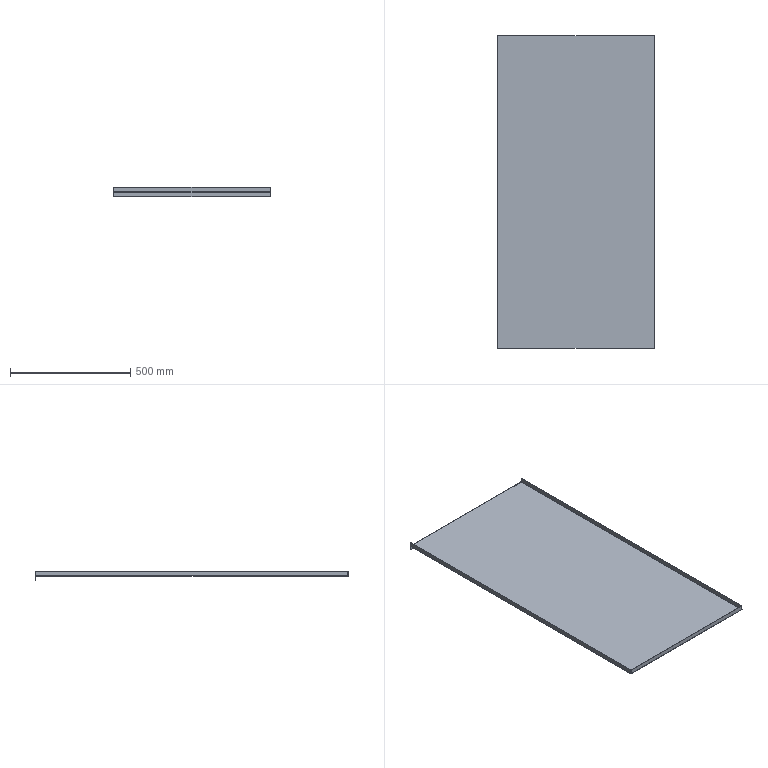Part | SolidWorks | 1 solid | 38 faces | box 655.001 x 1302 x 38.5 mm | volume 1385254 mm3 | plane 26 | cylinder 8 | spline 4 | commonest cylinder face diameters 0.2 x4 3.2 x4
STEP:
#1=CARTESIAN_POINT('',(325.9,-649.4,-1.5));
#2=VERTEX_POINT('',#1);
#3=CARTESIAN_POINT('',(-325.9,-649.4,-1.5));
#4=VERTEX_POINT('',#3);
#5=CARTESIAN_POINT('',(325.9,-649.4,-1.5));
#6=DIRECTION('',(-1.,0.,0.));
#7=VECTOR('',#6,1000.);
#8=LINE('',#5,#7);
#9=EDGE_CURVE('',#2,#4,#8,.T.);
#10=ORIENTED_EDGE('',*,*,#9,.T.);
#11=CARTESIAN_POINT('',(-325.9,649.4,-1.5));
#12=VERTEX_POINT('',#11);
#13=CARTESIAN_POINT('',(-325.9,-649.4,-1.5));
#14=DIRECTION('',(0.,1.,0.));
#15=VECTOR('',#14,1000.);
#16=LINE('',#13,#15);
#17=EDGE_CURVE('',#4,#12,#16,.T.);
#18=ORIENTED_EDGE('',*,*,#17,.T.);
#19=CARTESIAN_POINT('',(325.9,649.4,-1.5));
#20=VERTEX_POINT('',#19);
#21=CARTESIAN_POINT('',(325.9,649.4,-1.5));
#22=DIRECTION('',(-1.,0.,0.));
#23=VECTOR('',#22,1000.);
#24=LINE('',#21,#23);
#25=EDGE_CURVE('',#20,#12,#24,.T.);
#26=ORIENTED_EDGE('',*,*,#25,.F.);
#27=CARTESIAN_POINT('',(325.9,649.4,-1.5));
#28=DIRECTION('',(0.,-1.,0.));
#29=VECTOR('',#28,1000.);
#30=LINE('',#27,#29);
#31=EDGE_CURVE('',#20,#2,#30,.T.);
#32=ORIENTED_EDGE('',*,*,#31,.T.);
#33=EDGE_LOOP('',(#10,#18,#26,#32));
#34=FACE_OUTER_BOUND('',#33,.T.);
#35=CARTESIAN_POINT('',(0.,0.,-1.5));
#36=DIRECTION('',(0.,0.,1.));
#37=DIRECTION('',(1.,0.,0.));
#38=AXIS2_PLACEMENT_3D('',#35,#36,#37);
#39=PLANE('',#38);
#40=ADVANCED_FACE('',(#34),#39,.F.);
#41=CARTESIAN_POINT('',(-325.9,-649.4,0.));
#42=VERTEX_POINT('',#41);
#43=CARTESIAN_POINT('',(-325.9,649.4,0.));
#44=VERTEX_POINT('',#43);
#45=CARTESIAN_POINT('',(-325.9,-649.4,0.));
#46=DIRECTION('',(0.,1.,0.));
#47=VECTOR('',#46,1000.);
#48=LINE('',#45,#47);
#49=EDGE_CURVE('',#42,#44,#48,.T.);
#50=ORIENTED_EDGE('',*,*,#49,.F.);
#51=CARTESIAN_POINT('',(325.9,-649.4,0.));
#52=VERTEX_POINT('',#51);
#53=CARTESIAN_POINT('',(325.9,-649.4,0.));
#54=DIRECTION('',(-1.,0.,0.));
#55=VECTOR('',#54,1000.);
#56=LINE('',#53,#55);
#57=EDGE_CURVE('',#52,#42,#56,.T.);
#58=ORIENTED_EDGE('',*,*,#57,.F.);
#59=CARTESIAN_POINT('',(325.9,649.4,0.));
#60=VERTEX_POINT('',#59);
#61=CARTESIAN_POINT('',(325.9,649.4,0.));
#62=DIRECTION('',(0.,-1.,0.));
#63=VECTOR('',#62,1000.);
#64=LINE('',#61,#63);
#65=EDGE_CURVE('',#60,#52,#64,.T.);
#66=ORIENTED_EDGE('',*,*,#65,.F.);
#67=CARTESIAN_POINT('',(325.9,649.4,0.));
#68=DIRECTION('',(-1.,0.,0.));
#69=VECTOR('',#68,1000.);
#70=LINE('',#67,#69);
#71=EDGE_CURVE('',#60,#44,#70,.T.);
#72=ORIENTED_EDGE('',*,*,#71,.T.);
#73=EDGE_LOOP('',(#50,#58,#66,#72));
#74=FACE_OUTER_BOUND('',#73,.T.);
#75=CARTESIAN_POINT('',(0.,0.,0.));
#76=DIRECTION('',(0.,0.,1.));
#77=DIRECTION('',(1.,0.,0.));
#78=AXIS2_PLACEMENT_3D('',#75,#76,#77);
#79=PLANE('',#78);
#80=ADVANCED_FACE('',(#74),#79,.T.);
#81=CARTESIAN_POINT('',(-327.5,649.4,0.1));
#82=VERTEX_POINT('',#81);
#83=CARTESIAN_POINT('',(-326.,649.4,0.1));
#84=VERTEX_POINT('',#83);
#85=CARTESIAN_POINT('',(-326.,649.4,0.1));
#86=DIRECTION('',(1.,0.,0.));
#87=VECTOR('',#86,1000.);
#88=LINE('',#85,#87);
#89=EDGE_CURVE('',#82,#84,#88,.T.);
#90=ORIENTED_EDGE('',*,*,#89,.T.);
#91=CARTESIAN_POINT('',(-325.9,649.4,0.1));
#92=DIRECTION('',(0.,1.,0.));
#93=DIRECTION('',(0.,0.,-1.));
#94=AXIS2_PLACEMENT_3D('',#91,#92,#93);
#95=CIRCLE('',#94,0.1);
#96=EDGE_CURVE('',#44,#84,#95,.T.);
#97=ORIENTED_EDGE('',*,*,#96,.F.);
#98=CARTESIAN_POINT('',(-325.9,649.4,0.));
#99=DIRECTION('',(0.,0.,-1.));
#100=VECTOR('',#99,1000.);
#101=LINE('',#98,#100);
#102=EDGE_CURVE('',#44,#12,#101,.T.);
#103=ORIENTED_EDGE('',*,*,#102,.T.);
#104=CARTESIAN_POINT('',(-325.9,649.4,0.1));
#105=DIRECTION('',(0.,1.,0.));
#106=DIRECTION('',(0.,0.,-1.));
#107=AXIS2_PLACEMENT_3D('',#104,#105,#106);
#108=CIRCLE('',#107,1.6);
#109=EDGE_CURVE('',#12,#82,#108,.T.);
#110=ORIENTED_EDGE('',*,*,#109,.T.);
#111=EDGE_LOOP('',(#90,#97,#103,#110));
#112=FACE_OUTER_BOUND('',#111,.T.);
#113=CARTESIAN_POINT('',(-325.9,649.4,0.1));
#114=DIRECTION('',(0.,1.,0.));
#115=DIRECTION('',(0.,0.,1.));
#116=AXIS2_PLACEMENT_3D('',#113,#114,#115);
#117=PLANE('',#116);
#118=ADVANCED_FACE('',(#112),#117,.T.);
#119=CARTESIAN_POINT('',(-326.,-648.793,0.1));
#120=VERTEX_POINT('',#119);
#121=CARTESIAN_POINT('',(-326.,-648.793,0.1));
#122=CARTESIAN_POINT('',(-326.,-648.894,0.07382));
#123=CARTESIAN_POINT('',(-325.989,-648.995,0.0478));
#124=CARTESIAN_POINT('',(-325.952,-649.198,0.01078));
#125=CARTESIAN_POINT('',(-325.926,-649.299,0.));
#126=CARTESIAN_POINT('',(-325.9,-649.4,0.));
#127=B_SPLINE_CURVE_WITH_KNOTS('',3,(#121,#122,#123,#124,#125,#126),.UNSPECIFIED.,.F.,.F.,(4,2,4),(0.,0.5,1.),.UNSPECIFIED.);
#128=EDGE_CURVE('',#120,#42,#127,.T.);
#129=ORIENTED_EDGE('',*,*,#128,.F.);
#130=CARTESIAN_POINT('',(-327.5,-648.793,0.1));
#131=VERTEX_POINT('',#130);
#132=CARTESIAN_POINT('',(-326.,-648.793,0.1));
#133=DIRECTION('',(1.,0.,0.));
#134=VECTOR('',#133,1000.);
#135=LINE('',#132,#134);
#136=EDGE_CURVE('',#131,#120,#135,.T.);
#137=ORIENTED_EDGE('',*,*,#136,.F.);
#138=CARTESIAN_POINT('',(-327.5,-648.793,0.1));
#139=CARTESIAN_POINT('',(-327.5,-648.844,-0.1115));
#140=CARTESIAN_POINT('',(-327.46,-648.893,-0.3151));
#141=CARTESIAN_POINT('',(-327.299,-648.995,-0.7048));
#142=CARTESIAN_POINT('',(-327.181,-649.045,-0.881));
#143=CARTESIAN_POINT('',(-326.958,-649.121,-1.105));
#144=CARTESIAN_POINT('',(-326.878,-649.147,-1.171));
#145=CARTESIAN_POINT('',(-326.704,-649.197,-1.287));
#146=CARTESIAN_POINT('',(-326.61,-649.223,-1.338));
#147=CARTESIAN_POINT('',(-326.32,-649.299,-1.458));
#148=CARTESIAN_POINT('',(-326.112,-649.349,-1.5));
#149=CARTESIAN_POINT('',(-325.9,-649.4,-1.5));
#150=B_SPLINE_CURVE_WITH_KNOTS('',3,(#138,#139,#140,#141,#142,#143,#144,#145,#146,#147,#148,#149),.UNSPECIFIED.,.F.,.F.,(4,2,2,2,2,4),(0.,0.0006399,0.00128,0.0016,0.00192,0.00256),.UNSPECIFIED.);
#151=EDGE_CURVE('',#131,#4,#150,.T.);
#152=ORIENTED_EDGE('',*,*,#151,.T.);
#153=CARTESIAN_POINT('',(-325.9,-649.4,0.));
#154=DIRECTION('',(0.,0.,-1.));
#155=VECTOR('',#154,1000.);
#156=LINE('',#153,#155);
#157=EDGE_CURVE('',#42,#4,#156,.T.);
#158=ORIENTED_EDGE('',*,*,#157,.F.);
#159=EDGE_LOOP('',(#129,#137,#152,#158));
#160=FACE_OUTER_BOUND('',#159,.T.);
#161=CARTESIAN_POINT('',(-327.515,-648.793,0.1));
#162=CARTESIAN_POINT('',(-327.515,-648.843,-0.1114));
#163=CARTESIAN_POINT('',(-327.473,-648.894,-0.3227));
#164=CARTESIAN_POINT('',(-327.311,-648.995,-0.7133));
#165=CARTESIAN_POINT('',(-327.191,-649.046,-0.8925));
#166=CARTESIAN_POINT('',(-326.892,-649.147,-1.191));
#167=CARTESIAN_POINT('',(-326.713,-649.198,-1.311));
#168=CARTESIAN_POINT('',(-326.323,-649.299,-1.473));
#169=CARTESIAN_POINT('',(-326.111,-649.349,-1.515));
#170=CARTESIAN_POINT('',(-325.9,-649.4,-1.515));
#171=CARTESIAN_POINT('',(-327.5,-648.793,0.1));
#172=CARTESIAN_POINT('',(-327.5,-648.843,-0.1095));
#173=CARTESIAN_POINT('',(-327.458,-648.894,-0.3188));
#174=CARTESIAN_POINT('',(-327.298,-648.995,-0.7058));
#175=CARTESIAN_POINT('',(-327.179,-649.046,-0.8833));
#176=CARTESIAN_POINT('',(-326.883,-649.147,-1.179));
#177=CARTESIAN_POINT('',(-326.706,-649.198,-1.298));
#178=CARTESIAN_POINT('',(-326.319,-649.299,-1.458));
#179=CARTESIAN_POINT('',(-326.109,-649.349,-1.5));
#180=CARTESIAN_POINT('',(-325.9,-649.4,-1.5));
#181=CARTESIAN_POINT('',(-326.,-648.793,0.1));
#182=CARTESIAN_POINT('',(-326.,-648.843,0.08691));
#183=CARTESIAN_POINT('',(-325.997,-648.894,0.07383));
#184=CARTESIAN_POINT('',(-325.987,-648.995,0.04964));
#185=CARTESIAN_POINT('',(-325.98,-649.046,0.03855));
#186=CARTESIAN_POINT('',(-325.961,-649.147,0.02003));
#187=CARTESIAN_POINT('',(-325.95,-649.198,0.01262));
#188=CARTESIAN_POINT('',(-325.926,-649.299,0.002603));
#189=CARTESIAN_POINT('',(-325.913,-649.349,0.));
#190=CARTESIAN_POINT('',(-325.9,-649.4,0.));
#191=B_SPLINE_SURFACE_WITH_KNOTS('',1,3,((#161,#162,#163,#164,#165,#166,#167,#168,#169,#170),(#171,#172,#173,#174,#175,#176,#177,#178,#179,#180),(#181,#182,#183,#184,#185,#186,#187,#188,#189,#190)),.UNSPECIFIED.,.F.,.F.,.F.,(2,1,2),(4,2,2,2,4),(-0.01,0.,1.),(0.,0.25,0.5,0.75,1.),.UNSPECIFIED.);
#192=ADVANCED_FACE('',(#160),#191,.F.);
#193=ORIENTED_EDGE('',*,*,#17,.F.);
#194=ORIENTED_EDGE('',*,*,#151,.F.);
#195=CARTESIAN_POINT('',(-327.5,651.,0.1));
#196=DIRECTION('',(0.,1.,0.));
#197=VECTOR('',#196,1000.);
#198=LINE('',#195,#197);
#199=EDGE_CURVE('',#131,#82,#198,.T.);
#200=ORIENTED_EDGE('',*,*,#199,.T.);
#201=ORIENTED_EDGE('',*,*,#109,.F.);
#202=EDGE_LOOP('',(#193,#194,#200,#201));
#203=FACE_OUTER_BOUND('',#202,.T.);
#204=CARTESIAN_POINT('',(-325.9,-649.4,0.1));
#205=DIRECTION('',(0.,-1.,0.));
#206=DIRECTION('',(-1.,0.,0.));
#207=AXIS2_PLACEMENT_3D('',#204,#205,#206);
#208=CYLINDRICAL_SURFACE('',#207,1.6);
#209=ADVANCED_FACE('',(#203),#208,.T.);
#210=ORIENTED_EDGE('',*,*,#49,.T.);
#211=ORIENTED_EDGE('',*,*,#96,.T.);
#212=CARTESIAN_POINT('',(-326.,651.,0.1));
#213=DIRECTION('',(0.,-1.,0.));
#214=VECTOR('',#213,1000.);
#215=LINE('',#212,#214);
#216=EDGE_CURVE('',#84,#120,#215,.T.);
#217=ORIENTED_EDGE('',*,*,#216,.T.);
#218=ORIENTED_EDGE('',*,*,#128,.T.);
#219=EDGE_LOOP('',(#210,#211,#217,#218));
#220=FACE_OUTER_BOUND('',#219,.T.);
#221=CARTESIAN_POINT('',(-325.9,-649.4,0.1));
#222=DIRECTION('',(0.,-1.,0.));
#223=DIRECTION('',(-1.,0.,0.));
#224=AXIS2_PLACEMENT_3D('',#221,#222,#223);
#225=CYLINDRICAL_SURFACE('',#224,0.1);
#226=ADVANCED_FACE('',(#220),#225,.F.);
#227=CARTESIAN_POINT('',(-327.5,649.4,18.5));
#228=VERTEX_POINT('',#227);
#229=CARTESIAN_POINT('',(-327.5,649.4,0.));
#230=DIRECTION('',(0.,0.,1.));
#231=VECTOR('',#230,1000.);
#232=LINE('',#229,#231);
#233=EDGE_CURVE('',#82,#228,#232,.T.);
#234=ORIENTED_EDGE('',*,*,#233,.T.);
#235=CARTESIAN_POINT('',(-326.,649.4,18.5));
#236=VERTEX_POINT('',#235);
#237=CARTESIAN_POINT('',(-326.,649.4,18.5));
#238=DIRECTION('',(1.,0.,0.));
#239=VECTOR('',#238,1000.);
#240=LINE('',#237,#239);
#241=EDGE_CURVE('',#228,#236,#240,.T.);
#242=ORIENTED_EDGE('',*,*,#241,.T.);
#243=CARTESIAN_POINT('',(-326.,649.4,0.));
#244=DIRECTION('',(0.,0.,1.));
#245=VECTOR('',#244,1000.);
#246=LINE('',#243,#245);
#247=EDGE_CURVE('',#84,#236,#246,.T.);
#248=ORIENTED_EDGE('',*,*,#247,.F.);
#249=ORIENTED_EDGE('',*,*,#89,.F.);
#250=EDGE_LOOP('',(#234,#242,#248,#249));
#251=FACE_OUTER_BOUND('',#250,.T.);
#252=CARTESIAN_POINT('',(-326.,649.4,0.));
#253=DIRECTION('',(0.,1.,0.));
#254=DIRECTION('',(0.,0.,1.));
#255=AXIS2_PLACEMENT_3D('',#252,#253,#254);
#256=PLANE('',#255);
#257=ADVANCED_FACE('',(#251),#256,.T.);
#258=ORIENTED_EDGE('',*,*,#199,.F.);
#259=CARTESIAN_POINT('',(-327.5,-648.793,18.5));
#260=VERTEX_POINT('',#259);
#261=CARTESIAN_POINT('',(-327.5,-648.793,0.));
#262=DIRECTION('',(0.,0.,1.));
#263=VECTOR('',#262,1000.);
#264=LINE('',#261,#263);
#265=EDGE_CURVE('',#131,#260,#264,.T.);
#266=ORIENTED_EDGE('',*,*,#265,.T.);
#267=CARTESIAN_POINT('',(-327.5,0.,18.5));
#268=DIRECTION('',(0.,1.,0.));
#269=VECTOR('',#268,1000.);
#270=LINE('',#267,#269);
#271=EDGE_CURVE('',#260,#228,#270,.T.);
#272=ORIENTED_EDGE('',*,*,#271,.T.);
#273=ORIENTED_EDGE('',*,*,#233,.F.);
#274=EDGE_LOOP('',(#258,#266,#272,#273));
#275=FACE_OUTER_BOUND('',#274,.T.);
#276=CARTESIAN_POINT('',(-327.5,0.,0.));
#277=DIRECTION('',(1.,0.,0.));
#278=DIRECTION('',(0.,0.,-1.));
#279=AXIS2_PLACEMENT_3D('',#276,#277,#278);
#280=PLANE('',#279);
#281=ADVANCED_FACE('',(#275),#280,.F.);
#282=CARTESIAN_POINT('',(-326.,-648.793,18.5));
#283=VERTEX_POINT('',#282);
#284=CARTESIAN_POINT('',(-326.,-648.793,0.));
#285=DIRECTION('',(0.,0.,1.));
#286=VECTOR('',#285,1000.);
#287=LINE('',#284,#286);
#288=EDGE_CURVE('',#120,#283,#287,.T.);
#289=ORIENTED_EDGE('',*,*,#288,.F.);
#290=ORIENTED_EDGE('',*,*,#216,.F.);
#291=ORIENTED_EDGE('',*,*,#247,.T.);
#292=CARTESIAN_POINT('',(-326.,651.,18.5));
#293=DIRECTION('',(0.,1.,0.));
#294=VECTOR('',#293,1000.);
#295=LINE('',#292,#294);
#296=EDGE_CURVE('',#283,#236,#295,.T.);
#297=ORIENTED_EDGE('',*,*,#296,.F.);
#298=EDGE_LOOP('',(#289,#290,#291,#297));
#299=FACE_OUTER_BOUND('',#298,.T.);
#300=CARTESIAN_POINT('',(-326.,0.,0.));
#301=DIRECTION('',(1.,0.,0.));
#302=DIRECTION('',(0.,0.,-1.));
#303=AXIS2_PLACEMENT_3D('',#300,#301,#302);
#304=PLANE('',#303);
#305=ADVANCED_FACE('',(#299),#304,.T.);
#306=ORIENTED_EDGE('',*,*,#271,.F.);
#307=CARTESIAN_POINT('',(-327.5,-648.793,18.5));
#308=DIRECTION('',(1.,0.,0.));
#309=VECTOR('',#308,1000.);
#310=LINE('',#307,#309);
#311=EDGE_CURVE('',#260,#283,#310,.T.);
#312=ORIENTED_EDGE('',*,*,#311,.T.);
#313=ORIENTED_EDGE('',*,*,#296,.T.);
#314=ORIENTED_EDGE('',*,*,#241,.F.);
#315=EDGE_LOOP('',(#306,#312,#313,#314));
#316=FACE_OUTER_BOUND('',#315,.T.);
#317=CARTESIAN_POINT('',(-327.5,651.,18.5));
#318=DIRECTION('',(0.,0.,-1.));
#319=DIRECTION('',(-1.,0.,0.));
#320=AXIS2_PLACEMENT_3D('',#317,#318,#319);
#321=PLANE('',#320);
#322=ADVANCED_FACE('',(#316),#321,.F.);
#323=ORIENTED_EDGE('',*,*,#311,.F.);
#324=ORIENTED_EDGE('',*,*,#265,.F.);
#325=ORIENTED_EDGE('',*,*,#136,.T.);
#326=ORIENTED_EDGE('',*,*,#288,.T.);
#327=EDGE_LOOP('',(#323,#324,#325,#326));
#328=FACE_OUTER_BOUND('',#327,.T.);
#329=CARTESIAN_POINT('',(-326.,-648.793,0.));
#330=DIRECTION('',(0.,1.,0.));
#331=DIRECTION('',(0.,0.,1.));
#332=AXIS2_PLACEMENT_3D('',#329,#330,#331);
#333=PLANE('',#332);
#334=ADVANCED_FACE('',(#328),#333,.F.);
#335=CARTESIAN_POINT('',(-325.9,651.,-1.6));
#336=VERTEX_POINT('',#335);
#337=CARTESIAN_POINT('',(-325.9,649.5,-1.6));
#338=VERTEX_POINT('',#337);
#339=CARTESIAN_POINT('',(-325.9,649.5,-1.6));
#340=DIRECTION('',(0.,-1.,0.));
#341=VECTOR('',#340,1000.);
#342=LINE('',#339,#341);
#343=EDGE_CURVE('',#336,#338,#342,.T.);
#344=ORIENTED_EDGE('',*,*,#343,.T.);
#345=CARTESIAN_POINT('',(-325.9,649.4,-1.6));
#346=DIRECTION('',(-1.,0.,0.));
#347=DIRECTION('',(0.,0.,-1.));
#348=AXIS2_PLACEMENT_3D('',#345,#346,#347);
#349=CIRCLE('',#348,0.1);
#350=EDGE_CURVE('',#12,#338,#349,.T.);
#351=ORIENTED_EDGE('',*,*,#350,.F.);
#352=ORIENTED_EDGE('',*,*,#102,.F.);
#353=CARTESIAN_POINT('',(-325.9,649.4,-1.6));
#354=DIRECTION('',(-1.,0.,0.));
#355=DIRECTION('',(0.,0.,-1.));
#356=AXIS2_PLACEMENT_3D('',#353,#354,#355);
#357=CIRCLE('',#356,1.6);
#358=EDGE_CURVE('',#44,#336,#357,.T.);
#359=ORIENTED_EDGE('',*,*,#358,.T.);
#360=EDGE_LOOP('',(#344,#351,#352,#359));
#361=FACE_OUTER_BOUND('',#360,.T.);
#362=CARTESIAN_POINT('',(-325.9,649.4,-1.6));
#363=DIRECTION('',(-1.,0.,0.));
#364=DIRECTION('',(0.,0.,1.));
#365=AXIS2_PLACEMENT_3D('',#362,#363,#364);
#366=PLANE('',#365);
#367=ADVANCED_FACE('',(#361),#366,.T.);
#368=CARTESIAN_POINT('',(325.9,649.5,-1.6));
#369=VERTEX_POINT('',#368);
#370=CARTESIAN_POINT('',(325.9,649.4,-1.6));
#371=DIRECTION('',(1.,0.,0.));
#372=DIRECTION('',(0.,0.,-1.));
#373=AXIS2_PLACEMENT_3D('',#370,#371,#372);
#374=CIRCLE('',#373,0.1);
#375=EDGE_CURVE('',#369,#20,#374,.T.);
#376=ORIENTED_EDGE('',*,*,#375,.F.);
#377=CARTESIAN_POINT('',(325.9,651.,-1.6));
#378=VERTEX_POINT('',#377);
#379=CARTESIAN_POINT('',(325.9,649.5,-1.6));
#380=DIRECTION('',(0.,-1.,0.));
#381=VECTOR('',#380,1000.);
#382=LINE('',#379,#381);
#383=EDGE_CURVE('',#378,#369,#382,.T.);
#384=ORIENTED_EDGE('',*,*,#383,.F.);
#385=CARTESIAN_POINT('',(325.9,649.4,-1.6));
#386=DIRECTION('',(1.,0.,0.));
#387=DIRECTION('',(0.,0.,-1.));
#388=AXIS2_PLACEMENT_3D('',#385,#386,#387);
#389=CIRCLE('',#388,1.6);
#390=EDGE_CURVE('',#378,#60,#389,.T.);
#391=ORIENTED_EDGE('',*,*,#390,.T.);
#392=CARTESIAN_POINT('',(325.9,649.4,-1.5));
#393=DIRECTION('',(0.,0.,1.));
#394=VECTOR('',#393,1000.);
#395=LINE('',#392,#394);
#396=EDGE_CURVE('',#20,#60,#395,.T.);
#397=ORIENTED_EDGE('',*,*,#396,.F.);
#398=EDGE_LOOP('',(#376,#384,#391,#397));
#399=FACE_OUTER_BOUND('',#398,.T.);
#400=CARTESIAN_POINT('',(325.9,649.4,-1.6));
#401=DIRECTION('',(-1.,0.,0.));
#402=DIRECTION('',(0.,0.,1.));
#403=AXIS2_PLACEMENT_3D('',#400,#401,#402);
#404=PLANE('',#403);
#405=ADVANCED_FACE('',(#399),#404,.F.);
#406=ORIENTED_EDGE('',*,*,#71,.F.);
#407=ORIENTED_EDGE('',*,*,#390,.F.);
#408=CARTESIAN_POINT('',(0.,651.,-1.6));
#409=DIRECTION('',(1.,0.,0.));
#410=VECTOR('',#409,1000.);
#411=LINE('',#408,#410);
#412=EDGE_CURVE('',#336,#378,#411,.T.);
#413=ORIENTED_EDGE('',*,*,#412,.F.);
#414=ORIENTED_EDGE('',*,*,#358,.F.);
#415=EDGE_LOOP('',(#406,#407,#413,#414));
#416=FACE_OUTER_BOUND('',#415,.T.);
#417=CARTESIAN_POINT('',(325.9,649.4,-1.6));
#418=DIRECTION('',(1.,0.,0.));
#419=DIRECTION('',(0.,1.,0.));
#420=AXIS2_PLACEMENT_3D('',#417,#418,#419);
#421=CYLINDRICAL_SURFACE('',#420,1.6);
#422=ADVANCED_FACE('',(#416),#421,.T.);
#423=ORIENTED_EDGE('',*,*,#25,.T.);
#424=ORIENTED_EDGE('',*,*,#350,.T.);
#425=CARTESIAN_POINT('',(-327.5,649.5,-1.6));
#426=DIRECTION('',(1.,0.,0.));
#427=VECTOR('',#426,1000.);
#428=LINE('',#425,#427);
#429=EDGE_CURVE('',#338,#369,#428,.T.);
#430=ORIENTED_EDGE('',*,*,#429,.T.);
#431=ORIENTED_EDGE('',*,*,#375,.T.);
#432=EDGE_LOOP('',(#423,#424,#430,#431));
#433=FACE_OUTER_BOUND('',#432,.T.);
#434=CARTESIAN_POINT('',(325.9,649.4,-1.6));
#435=DIRECTION('',(1.,0.,0.));
#436=DIRECTION('',(0.,1.,0.));
#437=AXIS2_PLACEMENT_3D('',#434,#435,#436);
#438=CYLINDRICAL_SURFACE('',#437,0.1);
#439=ADVANCED_FACE('',(#433),#438,.F.);
#440=CARTESIAN_POINT('',(-325.9,649.5,-20.));
#441=VERTEX_POINT('',#440);
#442=CARTESIAN_POINT('',(-325.9,651.,-20.));
#443=VERTEX_POINT('',#442);
#444=CARTESIAN_POINT('',(-325.9,651.,-20.));
#445=DIRECTION('',(0.,1.,0.));
#446=VECTOR('',#445,1000.);
#447=LINE('',#444,#446);
#448=EDGE_CURVE('',#441,#443,#447,.T.);
#449=ORIENTED_EDGE('',*,*,#448,.F.);
#450=CARTESIAN_POINT('',(-325.9,649.5,0.));
#451=DIRECTION('',(0.,0.,-1.));
#452=VECTOR('',#451,1000.);
#453=LINE('',#450,#452);
#454=EDGE_CURVE('',#338,#441,#453,.T.);
#455=ORIENTED_EDGE('',*,*,#454,.F.);
#456=ORIENTED_EDGE('',*,*,#343,.F.);
#457=CARTESIAN_POINT('',(-325.9,651.,0.));
#458=DIRECTION('',(0.,0.,1.));
#459=VECTOR('',#458,1000.);
#460=LINE('',#457,#459);
#461=EDGE_CURVE('',#443,#336,#460,.T.);
#462=ORIENTED_EDGE('',*,*,#461,.F.);
#463=EDGE_LOOP('',(#449,#455,#456,#462));
#464=FACE_OUTER_BOUND('',#463,.T.);
#465=CARTESIAN_POINT('',(-325.9,649.5,-1.5));
#466=DIRECTION('',(-1.,0.,0.));
#467=DIRECTION('',(0.,0.,1.));
#468=AXIS2_PLACEMENT_3D('',#465,#466,#467);
#469=PLANE('',#468);
#470=ADVANCED_FACE('',(#464),#469,.T.);
#471=CARTESIAN_POINT('',(325.9,651.,-20.));
#472=VERTEX_POINT('',#471);
#473=CARTESIAN_POINT('',(325.9,651.,-1.5));
#474=DIRECTION('',(0.,0.,1.));
#475=VECTOR('',#474,1000.);
#476=LINE('',#473,#475);
#477=EDGE_CURVE('',#472,#378,#476,.T.);
#478=ORIENTED_EDGE('',*,*,#477,.F.);
#479=CARTESIAN_POINT('',(327.5,651.,-20.));
#480=DIRECTION('',(1.,0.,0.));
#481=VECTOR('',#480,1000.);
#482=LINE('',#479,#481);
#483=EDGE_CURVE('',#443,#472,#482,.T.);
#484=ORIENTED_EDGE('',*,*,#483,.F.);
#485=ORIENTED_EDGE('',*,*,#461,.T.);
#486=ORIENTED_EDGE('',*,*,#412,.T.);
#487=EDGE_LOOP('',(#478,#484,#485,#486));
#488=FACE_OUTER_BOUND('',#487,.T.);
#489=CARTESIAN_POINT('',(0.,651.,0.));
#490=DIRECTION('',(0.,1.,0.));
#491=DIRECTION('',(-1.,0.,0.));
#492=AXIS2_PLACEMENT_3D('',#489,#490,#491);
#493=PLANE('',#492);
#494=ADVANCED_FACE('',(#488),#493,.T.);
#495=CARTESIAN_POINT('',(325.9,649.5,-20.));
#496=VERTEX_POINT('',#495);
#497=CARTESIAN_POINT('',(0.,649.5,-20.));
#498=DIRECTION('',(1.,0.,0.));
#499=VECTOR('',#498,1000.);
#500=LINE('',#497,#499);
#501=EDGE_CURVE('',#441,#496,#500,.T.);
#502=ORIENTED_EDGE('',*,*,#501,.T.);
#503=CARTESIAN_POINT('',(325.9,649.5,-1.5));
#504=DIRECTION('',(0.,0.,-1.));
#505=VECTOR('',#504,1000.);
#506=LINE('',#503,#505);
#507=EDGE_CURVE('',#369,#496,#506,.T.);
#508=ORIENTED_EDGE('',*,*,#507,.F.);
#509=ORIENTED_EDGE('',*,*,#429,.F.);
#510=ORIENTED_EDGE('',*,*,#454,.T.);
#511=EDGE_LOOP('',(#502,#508,#509,#510));
#512=FACE_OUTER_BOUND('',#511,.T.);
#513=CARTESIAN_POINT('',(0.,649.5,0.));
#514=DIRECTION('',(0.,1.,0.));
#515=DIRECTION('',(-1.,0.,0.));
#516=AXIS2_PLACEMENT_3D('',#513,#514,#515);
#517=PLANE('',#516);
#518=ADVANCED_FACE('',(#512),#517,.F.);
#519=CARTESIAN_POINT('',(325.9,649.5,-20.));
#520=DIRECTION('',(0.,1.,0.));
#521=VECTOR('',#520,1000.);
#522=LINE('',#519,#521);
#523=EDGE_CURVE('',#496,#472,#522,.T.);
#524=ORIENTED_EDGE('',*,*,#523,.F.);
#525=ORIENTED_EDGE('',*,*,#501,.F.);
#526=ORIENTED_EDGE('',*,*,#448,.T.);
#527=ORIENTED_EDGE('',*,*,#483,.T.);
#528=EDGE_LOOP('',(#524,#525,#526,#527));
#529=FACE_OUTER_BOUND('',#528,.T.);
#530=CARTESIAN_POINT('',(327.5,651.,-20.));
#531=DIRECTION('',(0.,0.,-1.));
#532=DIRECTION('',(0.,1.,0.));
#533=AXIS2_PLACEMENT_3D('',#530,#531,#532);
#534=PLANE('',#533);
#535=ADVANCED_FACE('',(#529),#534,.T.);
#536=ORIENTED_EDGE('',*,*,#507,.T.);
#537=ORIENTED_EDGE('',*,*,#523,.T.);
#538=ORIENTED_EDGE('',*,*,#477,.T.);
#539=ORIENTED_EDGE('',*,*,#383,.T.);
#540=EDGE_LOOP('',(#536,#537,#538,#539));
#541=FACE_OUTER_BOUND('',#540,.T.);
#542=CARTESIAN_POINT('',(325.9,649.5,-1.5));
#543=DIRECTION('',(-1.,0.,0.));
#544=DIRECTION('',(0.,0.,1.));
#545=AXIS2_PLACEMENT_3D('',#542,#543,#544);
#546=PLANE('',#545);
#547=ADVANCED_FACE('',(#541),#546,.F.);
#548=CARTESIAN_POINT('',(327.5,-648.793,0.1));
#549=VERTEX_POINT('',#548);
#550=CARTESIAN_POINT('',(326.,-648.793,0.1));
#551=VERTEX_POINT('',#550);
#552=CARTESIAN_POINT('',(326.,-648.793,0.1));
#553=DIRECTION('',(-1.,0.,0.));
#554=VECTOR('',#553,1000.);
#555=LINE('',#552,#554);
#556=EDGE_CURVE('',#549,#551,#555,.T.);
#557=ORIENTED_EDGE('',*,*,#556,.T.);
#558=CARTESIAN_POINT('',(325.9,-649.4,0.));
#559=CARTESIAN_POINT('',(325.926,-649.299,0.));
#560=CARTESIAN_POINT('',(325.952,-649.198,0.01078));
#561=CARTESIAN_POINT('',(325.989,-648.995,0.0478));
#562=CARTESIAN_POINT('',(326.,-648.894,0.07382));
#563=CARTESIAN_POINT('',(326.,-648.793,0.1));
#564=B_SPLINE_CURVE_WITH_KNOTS('',3,(#558,#559,#560,#561,#562,#563),.UNSPECIFIED.,.F.,.F.,(4,2,4),(0.,0.5,1.),.UNSPECIFIED.);
#565=EDGE_CURVE('',#52,#551,#564,.T.);
#566=ORIENTED_EDGE('',*,*,#565,.F.);
#567=CARTESIAN_POINT('',(325.9,-649.4,0.));
#568=DIRECTION('',(0.,0.,-1.));
#569=VECTOR('',#568,1000.);
#570=LINE('',#567,#569);
#571=EDGE_CURVE('',#52,#2,#570,.T.);
#572=ORIENTED_EDGE('',*,*,#571,.T.);
#573=CARTESIAN_POINT('',(325.9,-649.4,-1.5));
#574=CARTESIAN_POINT('',(326.112,-649.349,-1.5));
#575=CARTESIAN_POINT('',(326.315,-649.3,-1.46));
#576=CARTESIAN_POINT('',(326.705,-649.198,-1.299));
#577=CARTESIAN_POINT('',(326.881,-649.148,-1.181));
#578=CARTESIAN_POINT('',(327.105,-649.071,-0.9582));
#579=CARTESIAN_POINT('',(327.171,-649.046,-0.8775));
#580=CARTESIAN_POINT('',(327.287,-648.996,-0.7041));
#581=CARTESIAN_POINT('',(327.338,-648.97,-0.6103));
#582=CARTESIAN_POINT('',(327.458,-648.894,-0.32));
#583=CARTESIAN_POINT('',(327.5,-648.844,-0.1115));
#584=CARTESIAN_POINT('',(327.5,-648.793,0.1));
#585=B_SPLINE_CURVE_WITH_KNOTS('',3,(#573,#574,#575,#576,#577,#578,#579,#580,#581,#582,#583,#584),.UNSPECIFIED.,.F.,.F.,(4,2,2,2,2,4),(0.,0.0006399,0.00128,0.0016,0.00192,0.00256),.UNSPECIFIED.);
#586=EDGE_CURVE('',#2,#549,#585,.T.);
#587=ORIENTED_EDGE('',*,*,#586,.T.);
#588=EDGE_LOOP('',(#557,#566,#572,#587));
#589=FACE_OUTER_BOUND('',#588,.T.);
#590=CARTESIAN_POINT('',(325.9,-649.4,-1.515));
#591=CARTESIAN_POINT('',(326.111,-649.349,-1.515));
#592=CARTESIAN_POINT('',(326.323,-649.299,-1.473));
#593=CARTESIAN_POINT('',(326.713,-649.198,-1.311));
#594=CARTESIAN_POINT('',(326.892,-649.147,-1.191));
#595=CARTESIAN_POINT('',(327.191,-649.046,-0.8925));
#596=CARTESIAN_POINT('',(327.311,-648.995,-0.7133));
#597=CARTESIAN_POINT('',(327.473,-648.894,-0.3227));
#598=CARTESIAN_POINT('',(327.515,-648.843,-0.1114));
#599=CARTESIAN_POINT('',(327.515,-648.793,0.1));
#600=CARTESIAN_POINT('',(325.9,-649.4,-1.5));
#601=CARTESIAN_POINT('',(326.109,-649.349,-1.5));
#602=CARTESIAN_POINT('',(326.319,-649.299,-1.458));
#603=CARTESIAN_POINT('',(326.706,-649.198,-1.298));
#604=CARTESIAN_POINT('',(326.883,-649.147,-1.179));
#605=CARTESIAN_POINT('',(327.179,-649.046,-0.8833));
#606=CARTESIAN_POINT('',(327.298,-648.995,-0.7058));
#607=CARTESIAN_POINT('',(327.458,-648.894,-0.3188));
#608=CARTESIAN_POINT('',(327.5,-648.843,-0.1095));
#609=CARTESIAN_POINT('',(327.5,-648.793,0.1));
#610=CARTESIAN_POINT('',(325.9,-649.4,0.));
#611=CARTESIAN_POINT('',(325.913,-649.349,0.));
#612=CARTESIAN_POINT('',(325.926,-649.299,0.002603));
#613=CARTESIAN_POINT('',(325.95,-649.198,0.01262));
#614=CARTESIAN_POINT('',(325.961,-649.147,0.02003));
#615=CARTESIAN_POINT('',(325.98,-649.046,0.03855));
#616=CARTESIAN_POINT('',(325.987,-648.995,0.04964));
#617=CARTESIAN_POINT('',(325.997,-648.894,0.07383));
#618=CARTESIAN_POINT('',(326.,-648.843,0.08691));
#619=CARTESIAN_POINT('',(326.,-648.793,0.1));
#620=B_SPLINE_SURFACE_WITH_KNOTS('',1,3,((#590,#591,#592,#593,#594,#595,#596,#597,#598,#599),(#600,#601,#602,#603,#604,#605,#606,#607,#608,#609),(#610,#611,#612,#613,#614,#615,#616,#617,#618,#619)),.UNSPECIFIED.,.F.,.F.,.F.,(2,1,2),(4,2,2,2,4),(-0.01,0.,1.),(0.,0.25,0.5,0.75,1.),.UNSPECIFIED.);
#621=ADVANCED_FACE('',(#589),#620,.F.);
#622=CARTESIAN_POINT('',(326.,649.4,0.1));
#623=VERTEX_POINT('',#622);
#624=CARTESIAN_POINT('',(325.9,649.4,0.1));
#625=DIRECTION('',(0.,1.,0.));
#626=DIRECTION('',(0.,0.,1.));
#627=AXIS2_PLACEMENT_3D('',#624,#625,#626);
#628=CIRCLE('',#627,0.1);
#629=EDGE_CURVE('',#623,#60,#628,.T.);
#630=ORIENTED_EDGE('',*,*,#629,.F.);
#631=CARTESIAN_POINT('',(327.5,649.4,0.1));
#632=VERTEX_POINT('',#631);
#633=CARTESIAN_POINT('',(326.,649.4,0.1));
#634=DIRECTION('',(-1.,0.,0.));
#635=VECTOR('',#634,1000.);
#636=LINE('',#633,#635);
#637=EDGE_CURVE('',#632,#623,#636,.T.);
#638=ORIENTED_EDGE('',*,*,#637,.F.);
#639=CARTESIAN_POINT('',(325.9,649.4,0.1));
#640=DIRECTION('',(0.,1.,0.));
#641=DIRECTION('',(0.,0.,1.));
#642=AXIS2_PLACEMENT_3D('',#639,#640,#641);
#643=CIRCLE('',#642,1.6);
#644=EDGE_CURVE('',#632,#20,#643,.T.);
#645=ORIENTED_EDGE('',*,*,#644,.T.);
#646=ORIENTED_EDGE('',*,*,#396,.T.);
#647=EDGE_LOOP('',(#630,#638,#645,#646));
#648=FACE_OUTER_BOUND('',#647,.T.);
#649=CARTESIAN_POINT('',(325.9,649.4,0.1));
#650=DIRECTION('',(0.,-1.,0.));
#651=DIRECTION('',(0.,0.,-1.));
#652=AXIS2_PLACEMENT_3D('',#649,#650,#651);
#653=PLANE('',#652);
#654=ADVANCED_FACE('',(#648),#653,.F.);
#655=ORIENTED_EDGE('',*,*,#31,.F.);
#656=ORIENTED_EDGE('',*,*,#644,.F.);
#657=CARTESIAN_POINT('',(327.5,-651.,0.1));
#658=DIRECTION('',(0.,-1.,0.));
#659=VECTOR('',#658,1000.);
#660=LINE('',#657,#659);
#661=EDGE_CURVE('',#632,#549,#660,.T.);
#662=ORIENTED_EDGE('',*,*,#661,.T.);
#663=ORIENTED_EDGE('',*,*,#586,.F.);
#664=EDGE_LOOP('',(#655,#656,#662,#663));
#665=FACE_OUTER_BOUND('',#664,.T.);
#666=CARTESIAN_POINT('',(325.9,649.4,0.1));
#667=DIRECTION('',(0.,1.,0.));
#668=DIRECTION('',(1.,0.,0.));
#669=AXIS2_PLACEMENT_3D('',#666,#667,#668);
#670=CYLINDRICAL_SURFACE('',#669,1.6);
#671=ADVANCED_FACE('',(#665),#670,.T.);
#672=ORIENTED_EDGE('',*,*,#65,.T.);
#673=ORIENTED_EDGE('',*,*,#565,.T.);
#674=CARTESIAN_POINT('',(326.,-651.,0.1));
#675=DIRECTION('',(0.,1.,0.));
#676=VECTOR('',#675,1000.);
#677=LINE('',#674,#676);
#678=EDGE_CURVE('',#551,#623,#677,.T.);
#679=ORIENTED_EDGE('',*,*,#678,.T.);
#680=ORIENTED_EDGE('',*,*,#629,.T.);
#681=EDGE_LOOP('',(#672,#673,#679,#680));
#682=FACE_OUTER_BOUND('',#681,.T.);
#683=CARTESIAN_POINT('',(325.9,649.4,0.1));
#684=DIRECTION('',(0.,1.,0.));
#685=DIRECTION('',(1.,0.,0.));
#686=AXIS2_PLACEMENT_3D('',#683,#684,#685);
#687=CYLINDRICAL_SURFACE('',#686,0.1);
#688=ADVANCED_FACE('',(#682),#687,.F.);
#689=CARTESIAN_POINT('',(327.5,-648.793,18.5));
#690=VERTEX_POINT('',#689);
#691=CARTESIAN_POINT('',(327.5,-648.793,0.));
#692=DIRECTION('',(0.,0.,1.));
#693=VECTOR('',#692,1000.);
#694=LINE('',#691,#693);
#695=EDGE_CURVE('',#549,#690,#694,.T.);
#696=ORIENTED_EDGE('',*,*,#695,.T.);
#697=CARTESIAN_POINT('',(326.,-648.793,18.5));
#698=VERTEX_POINT('',#697);
#699=CARTESIAN_POINT('',(326.,-648.793,18.5));
#700=DIRECTION('',(-1.,0.,0.));
#701=VECTOR('',#700,1000.);
#702=LINE('',#699,#701);
#703=EDGE_CURVE('',#690,#698,#702,.T.);
#704=ORIENTED_EDGE('',*,*,#703,.T.);
#705=CARTESIAN_POINT('',(326.,-648.793,0.));
#706=DIRECTION('',(0.,0.,1.));
#707=VECTOR('',#706,1000.);
#708=LINE('',#705,#707);
#709=EDGE_CURVE('',#551,#698,#708,.T.);
#710=ORIENTED_EDGE('',*,*,#709,.F.);
#711=ORIENTED_EDGE('',*,*,#556,.F.);
#712=EDGE_LOOP('',(#696,#704,#710,#711));
#713=FACE_OUTER_BOUND('',#712,.T.);
#714=CARTESIAN_POINT('',(326.,-648.793,0.));
#715=DIRECTION('',(0.,-1.,0.));
#716=DIRECTION('',(0.,0.,-1.));
#717=AXIS2_PLACEMENT_3D('',#714,#715,#716);
#718=PLANE('',#717);
#719=ADVANCED_FACE('',(#713),#718,.T.);
#720=ORIENTED_EDGE('',*,*,#661,.F.);
#721=CARTESIAN_POINT('',(327.5,649.4,18.5));
#722=VERTEX_POINT('',#721);
#723=CARTESIAN_POINT('',(327.5,649.4,0.));
#724=DIRECTION('',(0.,0.,1.));
#725=VECTOR('',#724,1000.);
#726=LINE('',#723,#725);
#727=EDGE_CURVE('',#632,#722,#726,.T.);
#728=ORIENTED_EDGE('',*,*,#727,.T.);
#729=CARTESIAN_POINT('',(327.5,0.,18.5));
#730=DIRECTION('',(0.,-1.,0.));
#731=VECTOR('',#730,1000.);
#732=LINE('',#729,#731);
#733=EDGE_CURVE('',#722,#690,#732,.T.);
#734=ORIENTED_EDGE('',*,*,#733,.T.);
#735=ORIENTED_EDGE('',*,*,#695,.F.);
#736=EDGE_LOOP('',(#720,#728,#734,#735));
#737=FACE_OUTER_BOUND('',#736,.T.);
#738=CARTESIAN_POINT('',(327.5,0.,0.));
#739=DIRECTION('',(-1.,0.,0.));
#740=DIRECTION('',(0.,0.,1.));
#741=AXIS2_PLACEMENT_3D('',#738,#739,#740);
#742=PLANE('',#741);
#743=ADVANCED_FACE('',(#737),#742,.F.);
#744=CARTESIAN_POINT('',(326.,649.4,18.5));
#745=VERTEX_POINT('',#744);
#746=CARTESIAN_POINT('',(326.,649.4,0.));
#747=DIRECTION('',(0.,0.,1.));
#748=VECTOR('',#747,1000.);
#749=LINE('',#746,#748);
#750=EDGE_CURVE('',#623,#745,#749,.T.);
#751=ORIENTED_EDGE('',*,*,#750,.F.);
#752=ORIENTED_EDGE('',*,*,#678,.F.);
#753=ORIENTED_EDGE('',*,*,#709,.T.);
#754=CARTESIAN_POINT('',(326.,-651.,18.5));
#755=DIRECTION('',(0.,-1.,0.));
#756=VECTOR('',#755,1000.);
#757=LINE('',#754,#756);
#758=EDGE_CURVE('',#745,#698,#757,.T.);
#759=ORIENTED_EDGE('',*,*,#758,.F.);
#760=EDGE_LOOP('',(#751,#752,#753,#759));
#761=FACE_OUTER_BOUND('',#760,.T.);
#762=CARTESIAN_POINT('',(326.,0.,0.));
#763=DIRECTION('',(-1.,0.,0.));
#764=DIRECTION('',(0.,0.,1.));
#765=AXIS2_PLACEMENT_3D('',#762,#763,#764);
#766=PLANE('',#765);
#767=ADVANCED_FACE('',(#761),#766,.T.);
#768=ORIENTED_EDGE('',*,*,#733,.F.);
#769=CARTESIAN_POINT('',(327.5,649.4,18.5));
#770=DIRECTION('',(-1.,0.,0.));
#771=VECTOR('',#770,1000.);
#772=LINE('',#769,#771);
#773=EDGE_CURVE('',#722,#745,#772,.T.);
#774=ORIENTED_EDGE('',*,*,#773,.T.);
#775=ORIENTED_EDGE('',*,*,#758,.T.);
#776=ORIENTED_EDGE('',*,*,#703,.F.);
#777=EDGE_LOOP('',(#768,#774,#775,#776));
#778=FACE_OUTER_BOUND('',#777,.T.);
#779=CARTESIAN_POINT('',(327.5,-651.,18.5));
#780=DIRECTION('',(0.,0.,-1.));
#781=DIRECTION('',(-1.,0.,0.));
#782=AXIS2_PLACEMENT_3D('',#779,#780,#781);
#783=PLANE('',#782);
#784=ADVANCED_FACE('',(#778),#783,.F.);
#785=ORIENTED_EDGE('',*,*,#773,.F.);
#786=ORIENTED_EDGE('',*,*,#727,.F.);
#787=ORIENTED_EDGE('',*,*,#637,.T.);
#788=ORIENTED_EDGE('',*,*,#750,.T.);
#789=EDGE_LOOP('',(#785,#786,#787,#788));
#790=FACE_OUTER_BOUND('',#789,.T.);
#791=CARTESIAN_POINT('',(326.,649.4,0.));
#792=DIRECTION('',(0.,-1.,0.));
#793=DIRECTION('',(0.,0.,-1.));
#794=AXIS2_PLACEMENT_3D('',#791,#792,#793);
#795=PLANE('',#794);
#796=ADVANCED_FACE('',(#790),#795,.F.);
#797=CARTESIAN_POINT('',(-325.293,-651.,0.1));
#798=VERTEX_POINT('',#797);
#799=CARTESIAN_POINT('',(-325.293,-649.5,0.1));
#800=VERTEX_POINT('',#799);
#801=CARTESIAN_POINT('',(-325.293,-649.5,0.1));
#802=DIRECTION('',(0.,1.,0.));
#803=VECTOR('',#802,1000.);
#804=LINE('',#801,#803);
#805=EDGE_CURVE('',#798,#800,#804,.T.);
#806=ORIENTED_EDGE('',*,*,#805,.T.);
#807=CARTESIAN_POINT('',(-325.9,-649.4,0.));
#808=CARTESIAN_POINT('',(-325.799,-649.426,0.));
#809=CARTESIAN_POINT('',(-325.698,-649.452,0.01078));
#810=CARTESIAN_POINT('',(-325.495,-649.489,0.0478));
#811=CARTESIAN_POINT('',(-325.394,-649.5,0.07382));
#812=CARTESIAN_POINT('',(-325.293,-649.5,0.1));
#813=B_SPLINE_CURVE_WITH_KNOTS('',3,(#807,#808,#809,#810,#811,#812),.UNSPECIFIED.,.F.,.F.,(4,2,4),(0.,0.5,1.),.UNSPECIFIED.);
#814=EDGE_CURVE('',#42,#800,#813,.T.);
#815=ORIENTED_EDGE('',*,*,#814,.F.);
#816=ORIENTED_EDGE('',*,*,#157,.T.);
#817=CARTESIAN_POINT('',(-325.9,-649.4,-1.5));
#818=CARTESIAN_POINT('',(-325.849,-649.612,-1.5));
#819=CARTESIAN_POINT('',(-325.8,-649.815,-1.46));
#820=CARTESIAN_POINT('',(-325.698,-650.205,-1.299));
#821=CARTESIAN_POINT('',(-325.648,-650.381,-1.181));
#822=CARTESIAN_POINT('',(-325.571,-650.605,-0.9582));
#823=CARTESIAN_POINT('',(-325.546,-650.671,-0.8775));
#824=CARTESIAN_POINT('',(-325.496,-650.787,-0.7041));
#825=CARTESIAN_POINT('',(-325.47,-650.838,-0.6103));
#826=CARTESIAN_POINT('',(-325.394,-650.958,-0.32));
#827=CARTESIAN_POINT('',(-325.344,-651.,-0.1115));
#828=CARTESIAN_POINT('',(-325.293,-651.,0.1));
#829=B_SPLINE_CURVE_WITH_KNOTS('',3,(#817,#818,#819,#820,#821,#822,#823,#824,#825,#826,#827,#828),.UNSPECIFIED.,.F.,.F.,(4,2,2,2,2,4),(0.,0.0006399,0.00128,0.0016,0.00192,0.00256),.UNSPECIFIED.);
#830=EDGE_CURVE('',#4,#798,#829,.T.);
#831=ORIENTED_EDGE('',*,*,#830,.T.);
#832=EDGE_LOOP('',(#806,#815,#816,#831));
#833=FACE_OUTER_BOUND('',#832,.T.);
#834=CARTESIAN_POINT('',(-325.9,-649.4,-1.515));
#835=CARTESIAN_POINT('',(-325.849,-649.611,-1.515));
#836=CARTESIAN_POINT('',(-325.799,-649.823,-1.473));
#837=CARTESIAN_POINT('',(-325.698,-650.213,-1.311));
#838=CARTESIAN_POINT('',(-325.647,-650.392,-1.191));
#839=CARTESIAN_POINT('',(-325.546,-650.691,-0.8925));
#840=CARTESIAN_POINT('',(-325.495,-650.811,-0.7133));
#841=CARTESIAN_POINT('',(-325.394,-650.973,-0.3227));
#842=CARTESIAN_POINT('',(-325.343,-651.015,-0.1114));
#843=CARTESIAN_POINT('',(-325.293,-651.015,0.1));
#844=CARTESIAN_POINT('',(-325.9,-649.4,-1.5));
#845=CARTESIAN_POINT('',(-325.849,-649.609,-1.5));
#846=CARTESIAN_POINT('',(-325.799,-649.819,-1.458));
#847=CARTESIAN_POINT('',(-325.698,-650.206,-1.298));
#848=CARTESIAN_POINT('',(-325.647,-650.383,-1.179));
#849=CARTESIAN_POINT('',(-325.546,-650.679,-0.8833));
#850=CARTESIAN_POINT('',(-325.495,-650.798,-0.7058));
#851=CARTESIAN_POINT('',(-325.394,-650.958,-0.3188));
#852=CARTESIAN_POINT('',(-325.343,-651.,-0.1095));
#853=CARTESIAN_POINT('',(-325.293,-651.,0.1));
#854=CARTESIAN_POINT('',(-325.9,-649.4,0.));
#855=CARTESIAN_POINT('',(-325.849,-649.413,0.));
#856=CARTESIAN_POINT('',(-325.799,-649.426,0.002603));
#857=CARTESIAN_POINT('',(-325.698,-649.45,0.01262));
#858=CARTESIAN_POINT('',(-325.647,-649.461,0.02003));
#859=CARTESIAN_POINT('',(-325.546,-649.48,0.03855));
#860=CARTESIAN_POINT('',(-325.495,-649.487,0.04964));
#861=CARTESIAN_POINT('',(-325.394,-649.497,0.07383));
#862=CARTESIAN_POINT('',(-325.343,-649.5,0.08691));
#863=CARTESIAN_POINT('',(-325.293,-649.5,0.1));
#864=B_SPLINE_SURFACE_WITH_KNOTS('',1,3,((#834,#835,#836,#837,#838,#839,#840,#841,#842,#843),(#844,#845,#846,#847,#848,#849,#850,#851,#852,#853),(#854,#855,#856,#857,#858,#859,#860,#861,#862,#863)),.UNSPECIFIED.,.F.,.F.,.F.,(2,1,2),(4,2,2,2,4),(-0.01,0.,1.),(0.,0.25,0.5,0.75,1.),.UNSPECIFIED.);
#865=ADVANCED_FACE('',(#833),#864,.F.);
#866=CARTESIAN_POINT('',(325.293,-649.5,0.1));
#867=VERTEX_POINT('',#866);
#868=CARTESIAN_POINT('',(325.293,-649.5,0.1));
#869=CARTESIAN_POINT('',(325.394,-649.5,0.07382));
#870=CARTESIAN_POINT('',(325.495,-649.489,0.0478));
#871=CARTESIAN_POINT('',(325.698,-649.452,0.01078));
#872=CARTESIAN_POINT('',(325.799,-649.426,0.));
#873=CARTESIAN_POINT('',(325.9,-649.4,0.));
#874=B_SPLINE_CURVE_WITH_KNOTS('',3,(#868,#869,#870,#871,#872,#873),.UNSPECIFIED.,.F.,.F.,(4,2,4),(0.,0.5,1.),.UNSPECIFIED.);
#875=EDGE_CURVE('',#867,#52,#874,.T.);
#876=ORIENTED_EDGE('',*,*,#875,.F.);
#877=CARTESIAN_POINT('',(325.293,-651.,0.1));
#878=VERTEX_POINT('',#877);
#879=CARTESIAN_POINT('',(325.293,-649.5,0.1));
#880=DIRECTION('',(0.,1.,0.));
#881=VECTOR('',#880,1000.);
#882=LINE('',#879,#881);
#883=EDGE_CURVE('',#878,#867,#882,.T.);
#884=ORIENTED_EDGE('',*,*,#883,.F.);
#885=CARTESIAN_POINT('',(325.293,-651.,0.1));
#886=CARTESIAN_POINT('',(325.344,-651.,-0.1115));
#887=CARTESIAN_POINT('',(325.393,-650.96,-0.3151));
#888=CARTESIAN_POINT('',(325.495,-650.799,-0.7048));
#889=CARTESIAN_POINT('',(325.545,-650.681,-0.881));
#890=CARTESIAN_POINT('',(325.621,-650.458,-1.105));
#891=CARTESIAN_POINT('',(325.647,-650.378,-1.171));
#892=CARTESIAN_POINT('',(325.697,-650.204,-1.287));
#893=CARTESIAN_POINT('',(325.723,-650.11,-1.338));
#894=CARTESIAN_POINT('',(325.799,-649.82,-1.458));
#895=CARTESIAN_POINT('',(325.849,-649.612,-1.5));
#896=CARTESIAN_POINT('',(325.9,-649.4,-1.5));
#897=B_SPLINE_CURVE_WITH_KNOTS('',3,(#885,#886,#887,#888,#889,#890,#891,#892,#893,#894,#895,#896),.UNSPECIFIED.,.F.,.F.,(4,2,2,2,2,4),(0.,0.0006399,0.00128,0.0016,0.00192,0.00256),.UNSPECIFIED.);
#898=EDGE_CURVE('',#878,#2,#897,.T.);
#899=ORIENTED_EDGE('',*,*,#898,.T.);
#900=ORIENTED_EDGE('',*,*,#571,.F.);
#901=EDGE_LOOP('',(#876,#884,#899,#900));
#902=FACE_OUTER_BOUND('',#901,.T.);
#903=CARTESIAN_POINT('',(325.293,-651.015,0.1));
#904=CARTESIAN_POINT('',(325.343,-651.015,-0.1114));
#905=CARTESIAN_POINT('',(325.394,-650.973,-0.3227));
#906=CARTESIAN_POINT('',(325.495,-650.811,-0.7133));
#907=CARTESIAN_POINT('',(325.546,-650.691,-0.8925));
#908=CARTESIAN_POINT('',(325.647,-650.392,-1.191));
#909=CARTESIAN_POINT('',(325.698,-650.213,-1.311));
#910=CARTESIAN_POINT('',(325.799,-649.823,-1.473));
#911=CARTESIAN_POINT('',(325.849,-649.611,-1.515));
#912=CARTESIAN_POINT('',(325.9,-649.4,-1.515));
#913=CARTESIAN_POINT('',(325.293,-651.,0.1));
#914=CARTESIAN_POINT('',(325.343,-651.,-0.1095));
#915=CARTESIAN_POINT('',(325.394,-650.958,-0.3188));
#916=CARTESIAN_POINT('',(325.495,-650.798,-0.7058));
#917=CARTESIAN_POINT('',(325.546,-650.679,-0.8833));
#918=CARTESIAN_POINT('',(325.647,-650.383,-1.179));
#919=CARTESIAN_POINT('',(325.698,-650.206,-1.298));
#920=CARTESIAN_POINT('',(325.799,-649.819,-1.458));
#921=CARTESIAN_POINT('',(325.849,-649.609,-1.5));
#922=CARTESIAN_POINT('',(325.9,-649.4,-1.5));
#923=CARTESIAN_POINT('',(325.293,-649.5,0.1));
#924=CARTESIAN_POINT('',(325.343,-649.5,0.08691));
#925=CARTESIAN_POINT('',(325.394,-649.497,0.07383));
#926=CARTESIAN_POINT('',(325.495,-649.487,0.04964));
#927=CARTESIAN_POINT('',(325.546,-649.48,0.03855));
#928=CARTESIAN_POINT('',(325.647,-649.461,0.02003));
#929=CARTESIAN_POINT('',(325.698,-649.45,0.01262));
#930=CARTESIAN_POINT('',(325.799,-649.426,0.002603));
#931=CARTESIAN_POINT('',(325.849,-649.413,0.));
#932=CARTESIAN_POINT('',(325.9,-649.4,0.));
#933=B_SPLINE_SURFACE_WITH_KNOTS('',1,3,((#903,#904,#905,#906,#907,#908,#909,#910,#911,#912),(#913,#914,#915,#916,#917,#918,#919,#920,#921,#922),(#923,#924,#925,#926,#927,#928,#929,#930,#931,#932)),.UNSPECIFIED.,.F.,.F.,.F.,(2,1,2),(4,2,2,2,4),(-0.01,0.,1.),(0.,0.25,0.5,0.75,1.),.UNSPECIFIED.);
#934=ADVANCED_FACE('',(#902),#933,.F.);
#935=ORIENTED_EDGE('',*,*,#9,.F.);
#936=ORIENTED_EDGE('',*,*,#898,.F.);
#937=CARTESIAN_POINT('',(-327.5,-651.,0.1));
#938=DIRECTION('',(-1.,0.,0.));
#939=VECTOR('',#938,1000.);
#940=LINE('',#937,#939);
#941=EDGE_CURVE('',#878,#798,#940,.T.);
#942=ORIENTED_EDGE('',*,*,#941,.T.);
#943=ORIENTED_EDGE('',*,*,#830,.F.);
#944=EDGE_LOOP('',(#935,#936,#942,#943));
#945=FACE_OUTER_BOUND('',#944,.T.);
#946=CARTESIAN_POINT('',(325.9,-649.4,0.1));
#947=DIRECTION('',(1.,0.,0.));
#948=DIRECTION('',(0.,-1.,0.));
#949=AXIS2_PLACEMENT_3D('',#946,#947,#948);
#950=CYLINDRICAL_SURFACE('',#949,1.6);
#951=ADVANCED_FACE('',(#945),#950,.T.);
#952=ORIENTED_EDGE('',*,*,#57,.T.);
#953=ORIENTED_EDGE('',*,*,#814,.T.);
#954=CARTESIAN_POINT('',(-327.5,-649.5,0.1));
#955=DIRECTION('',(1.,0.,0.));
#956=VECTOR('',#955,1000.);
#957=LINE('',#954,#956);
#958=EDGE_CURVE('',#800,#867,#957,.T.);
#959=ORIENTED_EDGE('',*,*,#958,.T.);
#960=ORIENTED_EDGE('',*,*,#875,.T.);
#961=EDGE_LOOP('',(#952,#953,#959,#960));
#962=FACE_OUTER_BOUND('',#961,.T.);
#963=CARTESIAN_POINT('',(325.9,-649.4,0.1));
#964=DIRECTION('',(1.,0.,0.));
#965=DIRECTION('',(0.,-1.,0.));
#966=AXIS2_PLACEMENT_3D('',#963,#964,#965);
#967=CYLINDRICAL_SURFACE('',#966,0.1);
#968=ADVANCED_FACE('',(#962),#967,.F.);
#969=CARTESIAN_POINT('',(-325.293,-651.,18.5));
#970=VERTEX_POINT('',#969);
#971=CARTESIAN_POINT('',(-325.293,-651.,0.));
#972=DIRECTION('',(0.,0.,1.));
#973=VECTOR('',#972,1000.);
#974=LINE('',#971,#973);
#975=EDGE_CURVE('',#798,#970,#974,.T.);
#976=ORIENTED_EDGE('',*,*,#975,.T.);
#977=CARTESIAN_POINT('',(-325.293,-649.5,18.5));
#978=VERTEX_POINT('',#977);
#979=CARTESIAN_POINT('',(-325.293,-649.5,18.5));
#980=DIRECTION('',(0.,1.,0.));
#981=VECTOR('',#980,1000.);
#982=LINE('',#979,#981);
#983=EDGE_CURVE('',#970,#978,#982,.T.);
#984=ORIENTED_EDGE('',*,*,#983,.T.);
#985=CARTESIAN_POINT('',(-325.293,-649.5,0.));
#986=DIRECTION('',(0.,0.,1.));
#987=VECTOR('',#986,1000.);
#988=LINE('',#985,#987);
#989=EDGE_CURVE('',#800,#978,#988,.T.);
#990=ORIENTED_EDGE('',*,*,#989,.F.);
#991=ORIENTED_EDGE('',*,*,#805,.F.);
#992=EDGE_LOOP('',(#976,#984,#990,#991));
#993=FACE_OUTER_BOUND('',#992,.T.);
#994=CARTESIAN_POINT('',(-325.293,-649.5,0.));
#995=DIRECTION('',(-1.,0.,0.));
#996=DIRECTION('',(0.,0.,1.));
#997=AXIS2_PLACEMENT_3D('',#994,#995,#996);
#998=PLANE('',#997);
#999=ADVANCED_FACE('',(#993),#998,.T.);
#1000=ORIENTED_EDGE('',*,*,#941,.F.);
#1001=CARTESIAN_POINT('',(325.293,-651.,18.5));
#1002=VERTEX_POINT('',#1001);
#1003=CARTESIAN_POINT('',(325.293,-651.,0.));
#1004=DIRECTION('',(0.,0.,1.));
#1005=VECTOR('',#1004,1000.);
#1006=LINE('',#1003,#1005);
#1007=EDGE_CURVE('',#878,#1002,#1006,.T.);
#1008=ORIENTED_EDGE('',*,*,#1007,.T.);
#1009=CARTESIAN_POINT('',(0.,-651.,18.5));
#1010=DIRECTION('',(-1.,0.,0.));
#1011=VECTOR('',#1010,1000.);
#1012=LINE('',#1009,#1011);
#1013=EDGE_CURVE('',#1002,#970,#1012,.T.);
#1014=ORIENTED_EDGE('',*,*,#1013,.T.);
#1015=ORIENTED_EDGE('',*,*,#975,.F.);
#1016=EDGE_LOOP('',(#1000,#1008,#1014,#1015));
#1017=FACE_OUTER_BOUND('',#1016,.T.);
#1018=CARTESIAN_POINT('',(0.,-651.,0.));
#1019=DIRECTION('',(0.,1.,0.));
#1020=DIRECTION('',(0.,0.,1.));
#1021=AXIS2_PLACEMENT_3D('',#1018,#1019,#1020);
#1022=PLANE('',#1021);
#1023=ADVANCED_FACE('',(#1017),#1022,.F.);
#1024=CARTESIAN_POINT('',(325.293,-649.5,18.5));
#1025=VERTEX_POINT('',#1024);
#1026=CARTESIAN_POINT('',(325.293,-649.5,0.));
#1027=DIRECTION('',(0.,0.,1.));
#1028=VECTOR('',#1027,1000.);
#1029=LINE('',#1026,#1028);
#1030=EDGE_CURVE('',#867,#1025,#1029,.T.);
#1031=ORIENTED_EDGE('',*,*,#1030,.F.);
#1032=ORIENTED_EDGE('',*,*,#958,.F.);
#1033=ORIENTED_EDGE('',*,*,#989,.T.);
#1034=CARTESIAN_POINT('',(-327.5,-649.5,18.5));
#1035=DIRECTION('',(-1.,0.,0.));
#1036=VECTOR('',#1035,1000.);
#1037=LINE('',#1034,#1036);
#1038=EDGE_CURVE('',#1025,#978,#1037,.T.);
#1039=ORIENTED_EDGE('',*,*,#1038,.F.);
#1040=EDGE_LOOP('',(#1031,#1032,#1033,#1039));
#1041=FACE_OUTER_BOUND('',#1040,.T.);
#1042=CARTESIAN_POINT('',(0.,-649.5,0.));
#1043=DIRECTION('',(0.,1.,0.));
#1044=DIRECTION('',(0.,0.,1.));
#1045=AXIS2_PLACEMENT_3D('',#1042,#1043,#1044);
#1046=PLANE('',#1045);
#1047=ADVANCED_FACE('',(#1041),#1046,.T.);
#1048=ORIENTED_EDGE('',*,*,#1013,.F.);
#1049=CARTESIAN_POINT('',(325.293,-651.,18.5));
#1050=DIRECTION('',(0.,1.,0.));
#1051=VECTOR('',#1050,1000.);
#1052=LINE('',#1049,#1051);
#1053=EDGE_CURVE('',#1002,#1025,#1052,.T.);
#1054=ORIENTED_EDGE('',*,*,#1053,.T.);
#1055=ORIENTED_EDGE('',*,*,#1038,.T.);
#1056=ORIENTED_EDGE('',*,*,#983,.F.);
#1057=EDGE_LOOP('',(#1048,#1054,#1055,#1056));
#1058=FACE_OUTER_BOUND('',#1057,.T.);
#1059=CARTESIAN_POINT('',(-327.5,-651.,18.5));
#1060=DIRECTION('',(0.,0.,-1.));
#1061=DIRECTION('',(0.,1.,0.));
#1062=AXIS2_PLACEMENT_3D('',#1059,#1060,#1061);
#1063=PLANE('',#1062);
#1064=ADVANCED_FACE('',(#1058),#1063,.F.);
#1065=ORIENTED_EDGE('',*,*,#1053,.F.);
#1066=ORIENTED_EDGE('',*,*,#1007,.F.);
#1067=ORIENTED_EDGE('',*,*,#883,.T.);
#1068=ORIENTED_EDGE('',*,*,#1030,.T.);
#1069=EDGE_LOOP('',(#1065,#1066,#1067,#1068));
#1070=FACE_OUTER_BOUND('',#1069,.T.);
#1071=CARTESIAN_POINT('',(325.293,-649.5,0.));
#1072=DIRECTION('',(-1.,0.,0.));
#1073=DIRECTION('',(0.,0.,1.));
#1074=AXIS2_PLACEMENT_3D('',#1071,#1072,#1073);
#1075=PLANE('',#1074);
#1076=ADVANCED_FACE('',(#1070),#1075,.F.);
#1077=CLOSED_SHELL('',(#40,#80,#118,#192,#209,#226,#257,#281,#305,#322,#334,#367,#405,#422,#439,#470,#494,#518,#535,#547,#621,#654,#671,#688,#719,#743,#767,#784,#796,#865,#934,#951,#968,#999,#1023,#1047,#1064,#1076));
#1078=MANIFOLD_SOLID_BREP('',#1077);
#1079=CARTESIAN_POINT('',(0.,0.,0.));
#1080=DIRECTION('',(0.,0.,1.));
#1081=DIRECTION('',(1.,0.,0.));
#1082=AXIS2_PLACEMENT_3D('',#1079,#1080,#1081);
#1083=(LENGTH_UNIT()NAMED_UNIT(*)SI_UNIT(.MILLI.,.METRE.));
#1084=UNCERTAINTY_MEASURE_WITH_UNIT(LENGTH_MEASURE(0.00001),#1083,'','');
#1085=(NAMED_UNIT(*)PLANE_ANGLE_UNIT()SI_UNIT($,.RADIAN.));
#1086=(NAMED_UNIT(*)SI_UNIT($,.STERADIAN.)SOLID_ANGLE_UNIT());
#1087=(GEOMETRIC_REPRESENTATION_CONTEXT(3)GLOBAL_UNCERTAINTY_ASSIGNED_CONTEXT((#1084))GLOBAL_UNIT_ASSIGNED_CONTEXT((#1083,#1085,#1086))REPRESENTATION_CONTEXT('',''));
#1088=ADVANCED_BREP_SHAPE_REPRESENTATION('',(#1078,#1082),#1087);